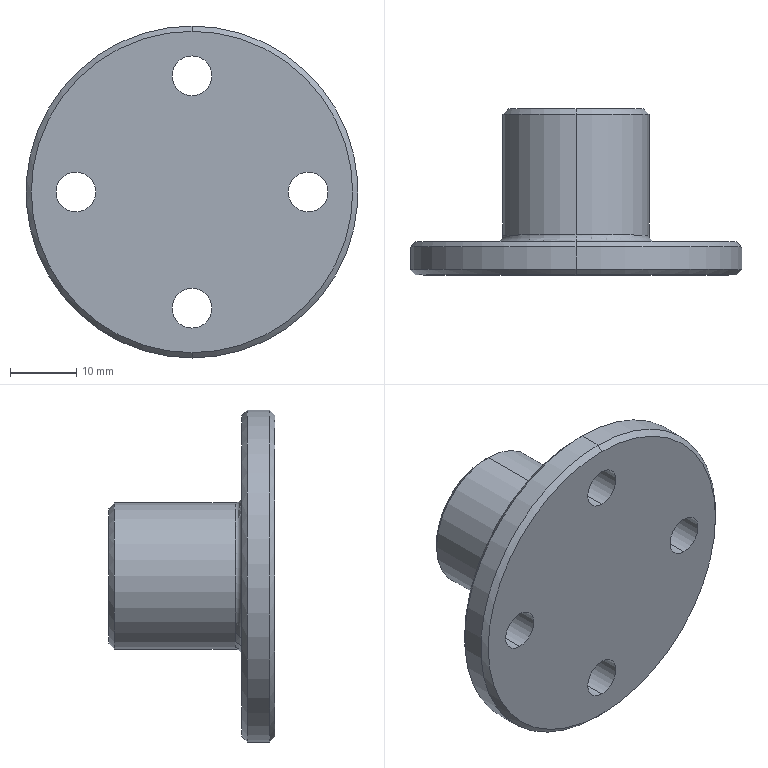Part | SolidWorks | features ICE 2, Chamfer 1, Extrusion 1, Fillet 1 | 1 solid | 28 faces | box 50 x 25 x 50 mm | volume 12711 mm3 | cylinder 14 | cone 8 | plane 4 | torus 2 | commonest cylinder face diameters 6 x8 16 x2 22 x2 50 x2
STEP:
#1=CARTESIAN_POINT('',(0.,6.,-11.));
#2=VERTEX_POINT('',#1);
#3=CARTESIAN_POINT('',(0.,6.,11.));
#4=VERTEX_POINT('',#3);
#5=CARTESIAN_POINT('',(0.,6.,0.));
#6=DIRECTION('',(0.,1.,0.));
#7=DIRECTION('',(0.,0.,1.));
#8=AXIS2_PLACEMENT_3D('',#5,#6,#7);
#9=CIRCLE('',#8,11.);
#10=EDGE_CURVE('',#2,#4,#9,.T.);
#11=ORIENTED_EDGE('',*,*,#10,.F.);
#12=CARTESIAN_POINT('',(0.,5.,-12.));
#13=VERTEX_POINT('',#12);
#14=CARTESIAN_POINT('',(0.,6.,-12.));
#15=DIRECTION('',(1.,0.,0.));
#16=DIRECTION('',(0.,0.,-1.));
#17=AXIS2_PLACEMENT_3D('',#14,#15,#16);
#18=CIRCLE('',#17,1.);
#19=EDGE_CURVE('',#2,#13,#18,.T.);
#20=ORIENTED_EDGE('',*,*,#19,.T.);
#21=CARTESIAN_POINT('',(0.,5.,12.));
#22=VERTEX_POINT('',#21);
#23=CARTESIAN_POINT('',(0.,5.,0.));
#24=DIRECTION('',(0.,-1.,0.));
#25=DIRECTION('',(0.,0.,1.));
#26=AXIS2_PLACEMENT_3D('',#23,#24,#25);
#27=CIRCLE('',#26,12.);
#28=EDGE_CURVE('',#22,#13,#27,.T.);
#29=ORIENTED_EDGE('',*,*,#28,.F.);
#30=CARTESIAN_POINT('',(0.,6.,12.));
#31=DIRECTION('',(-1.,0.,0.));
#32=DIRECTION('',(0.,0.,1.));
#33=AXIS2_PLACEMENT_3D('',#30,#31,#32);
#34=CIRCLE('',#33,1.);
#35=EDGE_CURVE('',#4,#22,#34,.T.);
#36=ORIENTED_EDGE('',*,*,#35,.F.);
#37=EDGE_LOOP('',(#11,#20,#29,#36));
#38=FACE_OUTER_BOUND('',#37,.T.);
#39=CARTESIAN_POINT('',(0.,6.,0.));
#40=DIRECTION('',(0.,1.,0.));
#41=DIRECTION('',(0.,0.,1.));
#42=AXIS2_PLACEMENT_3D('',#39,#40,#41);
#43=TOROIDAL_SURFACE('',#42,12.,1.);
#44=ADVANCED_FACE('',(#38),#43,.F.);
#45=CARTESIAN_POINT('',(0.,0.,-24.2));
#46=VERTEX_POINT('',#45);
#47=CARTESIAN_POINT('',(0.,0.,24.2));
#48=VERTEX_POINT('',#47);
#49=CARTESIAN_POINT('',(0.,0.,0.));
#50=DIRECTION('',(0.,-1.,0.));
#51=DIRECTION('',(0.,0.,1.));
#52=AXIS2_PLACEMENT_3D('',#49,#50,#51);
#53=CIRCLE('',#52,24.2);
#54=EDGE_CURVE('',#46,#48,#53,.T.);
#55=ORIENTED_EDGE('',*,*,#54,.F.);
#56=CARTESIAN_POINT('',(0.,0.8,-25.));
#57=VERTEX_POINT('',#56);
#58=CARTESIAN_POINT('',(0.,0.8,-25.));
#59=DIRECTION('',(0.,0.7071,-0.7071));
#60=VECTOR('',#59,1000.);
#61=LINE('',#58,#60);
#62=EDGE_CURVE('',#46,#57,#61,.T.);
#63=ORIENTED_EDGE('',*,*,#62,.T.);
#64=CARTESIAN_POINT('',(0.,0.8,25.));
#65=VERTEX_POINT('',#64);
#66=CARTESIAN_POINT('',(0.,0.8,0.));
#67=DIRECTION('',(0.,1.,0.));
#68=DIRECTION('',(0.,0.,1.));
#69=AXIS2_PLACEMENT_3D('',#66,#67,#68);
#70=CIRCLE('',#69,25.);
#71=EDGE_CURVE('',#65,#57,#70,.T.);
#72=ORIENTED_EDGE('',*,*,#71,.F.);
#73=CARTESIAN_POINT('',(0.,0.8,25.));
#74=DIRECTION('',(0.,0.7071,0.7071));
#75=VECTOR('',#74,1000.);
#76=LINE('',#73,#75);
#77=EDGE_CURVE('',#48,#65,#76,.T.);
#78=ORIENTED_EDGE('',*,*,#77,.F.);
#79=EDGE_LOOP('',(#55,#63,#72,#78));
#80=FACE_OUTER_BOUND('',#79,.T.);
#81=CARTESIAN_POINT('',(0.,0.8,0.));
#82=DIRECTION('',(0.,1.,0.));
#83=DIRECTION('',(0.,0.,1.));
#84=AXIS2_PLACEMENT_3D('',#81,#82,#83);
#85=CONICAL_SURFACE('',#84,25.,0.7854);
#86=ADVANCED_FACE('',(#80),#85,.T.);
#87=CARTESIAN_POINT('',(0.,5.,24.2));
#88=VERTEX_POINT('',#87);
#89=CARTESIAN_POINT('',(0.,5.,-24.2));
#90=VERTEX_POINT('',#89);
#91=CARTESIAN_POINT('',(0.,5.,0.));
#92=DIRECTION('',(0.,1.,0.));
#93=DIRECTION('',(0.,0.,1.));
#94=AXIS2_PLACEMENT_3D('',#91,#92,#93);
#95=CIRCLE('',#94,24.2);
#96=EDGE_CURVE('',#88,#90,#95,.T.);
#97=ORIENTED_EDGE('',*,*,#96,.F.);
#98=CARTESIAN_POINT('',(0.,4.2,25.));
#99=VERTEX_POINT('',#98);
#100=CARTESIAN_POINT('',(0.,5.,24.2));
#101=DIRECTION('',(0.,-0.7071,0.7071));
#102=VECTOR('',#101,1000.);
#103=LINE('',#100,#102);
#104=EDGE_CURVE('',#88,#99,#103,.T.);
#105=ORIENTED_EDGE('',*,*,#104,.T.);
#106=CARTESIAN_POINT('',(0.,4.2,-25.));
#107=VERTEX_POINT('',#106);
#108=CARTESIAN_POINT('',(0.,4.2,0.));
#109=DIRECTION('',(0.,-1.,0.));
#110=DIRECTION('',(0.,0.,1.));
#111=AXIS2_PLACEMENT_3D('',#108,#109,#110);
#112=CIRCLE('',#111,25.);
#113=EDGE_CURVE('',#107,#99,#112,.T.);
#114=ORIENTED_EDGE('',*,*,#113,.F.);
#115=CARTESIAN_POINT('',(0.,5.,-24.2));
#116=DIRECTION('',(0.,-0.7071,-0.7071));
#117=VECTOR('',#116,1000.);
#118=LINE('',#115,#117);
#119=EDGE_CURVE('',#90,#107,#118,.T.);
#120=ORIENTED_EDGE('',*,*,#119,.F.);
#121=EDGE_LOOP('',(#97,#105,#114,#120));
#122=FACE_OUTER_BOUND('',#121,.T.);
#123=CARTESIAN_POINT('',(0.,5.,0.));
#124=DIRECTION('',(0.,-1.,0.));
#125=DIRECTION('',(0.,0.,-1.));
#126=AXIS2_PLACEMENT_3D('',#123,#124,#125);
#127=CONICAL_SURFACE('',#126,24.2,0.7854);
#128=ADVANCED_FACE('',(#122),#127,.T.);
#129=CARTESIAN_POINT('',(0.,24.2,-8.));
#130=VERTEX_POINT('',#129);
#131=CARTESIAN_POINT('',(0.,24.2,8.));
#132=VERTEX_POINT('',#131);
#133=CARTESIAN_POINT('',(0.,24.2,0.));
#134=DIRECTION('',(0.,1.,0.));
#135=DIRECTION('',(0.,0.,1.));
#136=AXIS2_PLACEMENT_3D('',#133,#134,#135);
#137=CIRCLE('',#136,8.);
#138=EDGE_CURVE('',#130,#132,#137,.T.);
#139=ORIENTED_EDGE('',*,*,#138,.F.);
#140=CARTESIAN_POINT('',(0.,25.,-8.8));
#141=VERTEX_POINT('',#140);
#142=CARTESIAN_POINT('',(0.,24.2,-8.));
#143=DIRECTION('',(0.,0.7071,-0.7071));
#144=VECTOR('',#143,1000.);
#145=LINE('',#142,#144);
#146=EDGE_CURVE('',#130,#141,#145,.T.);
#147=ORIENTED_EDGE('',*,*,#146,.T.);
#148=CARTESIAN_POINT('',(0.,25.,8.8));
#149=VERTEX_POINT('',#148);
#150=CARTESIAN_POINT('',(0.,25.,0.));
#151=DIRECTION('',(0.,-1.,0.));
#152=DIRECTION('',(0.,0.,1.));
#153=AXIS2_PLACEMENT_3D('',#150,#151,#152);
#154=CIRCLE('',#153,8.8);
#155=EDGE_CURVE('',#149,#141,#154,.T.);
#156=ORIENTED_EDGE('',*,*,#155,.F.);
#157=CARTESIAN_POINT('',(0.,24.2,8.));
#158=DIRECTION('',(0.,0.7071,0.7071));
#159=VECTOR('',#158,1000.);
#160=LINE('',#157,#159);
#161=EDGE_CURVE('',#132,#149,#160,.T.);
#162=ORIENTED_EDGE('',*,*,#161,.F.);
#163=EDGE_LOOP('',(#139,#147,#156,#162));
#164=FACE_OUTER_BOUND('',#163,.T.);
#165=CARTESIAN_POINT('',(0.,24.2,0.));
#166=DIRECTION('',(0.,1.,0.));
#167=DIRECTION('',(0.,0.,1.));
#168=AXIS2_PLACEMENT_3D('',#165,#166,#167);
#169=CONICAL_SURFACE('',#168,8.,0.7854);
#170=ADVANCED_FACE('',(#164),#169,.F.);
#171=CARTESIAN_POINT('',(0.,25.,10.2));
#172=VERTEX_POINT('',#171);
#173=CARTESIAN_POINT('',(0.,25.,-10.2));
#174=VERTEX_POINT('',#173);
#175=CARTESIAN_POINT('',(0.,25.,0.));
#176=DIRECTION('',(0.,1.,0.));
#177=DIRECTION('',(0.,0.,1.));
#178=AXIS2_PLACEMENT_3D('',#175,#176,#177);
#179=CIRCLE('',#178,10.2);
#180=EDGE_CURVE('',#172,#174,#179,.T.);
#181=ORIENTED_EDGE('',*,*,#180,.F.);
#182=CARTESIAN_POINT('',(0.,24.2,11.));
#183=VERTEX_POINT('',#182);
#184=CARTESIAN_POINT('',(0.,25.,10.2));
#185=DIRECTION('',(0.,-0.7071,0.7071));
#186=VECTOR('',#185,1000.);
#187=LINE('',#184,#186);
#188=EDGE_CURVE('',#172,#183,#187,.T.);
#189=ORIENTED_EDGE('',*,*,#188,.T.);
#190=CARTESIAN_POINT('',(0.,24.2,-11.));
#191=VERTEX_POINT('',#190);
#192=CARTESIAN_POINT('',(0.,24.2,0.));
#193=DIRECTION('',(0.,-1.,0.));
#194=DIRECTION('',(0.,0.,1.));
#195=AXIS2_PLACEMENT_3D('',#192,#193,#194);
#196=CIRCLE('',#195,11.);
#197=EDGE_CURVE('',#191,#183,#196,.T.);
#198=ORIENTED_EDGE('',*,*,#197,.F.);
#199=CARTESIAN_POINT('',(0.,25.,-10.2));
#200=DIRECTION('',(0.,-0.7071,-0.7071));
#201=VECTOR('',#200,1000.);
#202=LINE('',#199,#201);
#203=EDGE_CURVE('',#174,#191,#202,.T.);
#204=ORIENTED_EDGE('',*,*,#203,.F.);
#205=EDGE_LOOP('',(#181,#189,#198,#204));
#206=FACE_OUTER_BOUND('',#205,.T.);
#207=CARTESIAN_POINT('',(0.,25.,0.));
#208=DIRECTION('',(0.,-1.,0.));
#209=DIRECTION('',(0.,0.,-1.));
#210=AXIS2_PLACEMENT_3D('',#207,#208,#209);
#211=CONICAL_SURFACE('',#210,10.2,0.7854);
#212=ADVANCED_FACE('',(#206),#211,.T.);
#213=ORIENTED_EDGE('',*,*,#138,.T.);
#214=CARTESIAN_POINT('',(0.,5.,8.));
#215=VERTEX_POINT('',#214);
#216=CARTESIAN_POINT('',(0.,25.,8.));
#217=DIRECTION('',(0.,-1.,0.));
#218=VECTOR('',#217,1000.);
#219=LINE('',#216,#218);
#220=EDGE_CURVE('',#132,#215,#219,.T.);
#221=ORIENTED_EDGE('',*,*,#220,.T.);
#222=CARTESIAN_POINT('',(0.,5.,-8.));
#223=VERTEX_POINT('',#222);
#224=CARTESIAN_POINT('',(0.,5.,0.));
#225=DIRECTION('',(0.,-1.,0.));
#226=DIRECTION('',(0.,0.,1.));
#227=AXIS2_PLACEMENT_3D('',#224,#225,#226);
#228=CIRCLE('',#227,8.);
#229=EDGE_CURVE('',#215,#223,#228,.T.);
#230=ORIENTED_EDGE('',*,*,#229,.T.);
#231=CARTESIAN_POINT('',(0.,25.,-8.));
#232=DIRECTION('',(0.,-1.,0.));
#233=VECTOR('',#232,1000.);
#234=LINE('',#231,#233);
#235=EDGE_CURVE('',#130,#223,#234,.T.);
#236=ORIENTED_EDGE('',*,*,#235,.F.);
#237=EDGE_LOOP('',(#213,#221,#230,#236));
#238=FACE_OUTER_BOUND('',#237,.T.);
#239=CARTESIAN_POINT('',(0.,25.,0.));
#240=DIRECTION('',(0.,-1.,0.));
#241=DIRECTION('',(0.,0.,-1.));
#242=AXIS2_PLACEMENT_3D('',#239,#240,#241);
#243=CYLINDRICAL_SURFACE('',#242,8.);
#244=ADVANCED_FACE('',(#238),#243,.F.);
#245=ORIENTED_EDGE('',*,*,#197,.T.);
#246=CARTESIAN_POINT('',(0.,25.,11.));
#247=DIRECTION('',(0.,-1.,0.));
#248=VECTOR('',#247,1000.);
#249=LINE('',#246,#248);
#250=EDGE_CURVE('',#183,#4,#249,.T.);
#251=ORIENTED_EDGE('',*,*,#250,.T.);
#252=CARTESIAN_POINT('',(0.,6.,0.));
#253=DIRECTION('',(0.,1.,0.));
#254=DIRECTION('',(0.,0.,1.));
#255=AXIS2_PLACEMENT_3D('',#252,#253,#254);
#256=CIRCLE('',#255,11.);
#257=EDGE_CURVE('',#4,#2,#256,.T.);
#258=ORIENTED_EDGE('',*,*,#257,.T.);
#259=CARTESIAN_POINT('',(0.,25.,-11.));
#260=DIRECTION('',(0.,-1.,0.));
#261=VECTOR('',#260,1000.);
#262=LINE('',#259,#261);
#263=EDGE_CURVE('',#191,#2,#262,.T.);
#264=ORIENTED_EDGE('',*,*,#263,.F.);
#265=EDGE_LOOP('',(#245,#251,#258,#264));
#266=FACE_OUTER_BOUND('',#265,.T.);
#267=CARTESIAN_POINT('',(0.,25.,0.));
#268=DIRECTION('',(0.,-1.,0.));
#269=DIRECTION('',(0.,0.,-1.));
#270=AXIS2_PLACEMENT_3D('',#267,#268,#269);
#271=CYLINDRICAL_SURFACE('',#270,11.);
#272=ADVANCED_FACE('',(#266),#271,.T.);
#273=CARTESIAN_POINT('',(-17.5,5.,-3.));
#274=VERTEX_POINT('',#273);
#275=CARTESIAN_POINT('',(-17.5,5.,3.));
#276=VERTEX_POINT('',#275);
#277=CARTESIAN_POINT('',(-17.5,5.,0.));
#278=DIRECTION('',(0.,1.,0.));
#279=DIRECTION('',(0.,0.,1.));
#280=AXIS2_PLACEMENT_3D('',#277,#278,#279);
#281=CIRCLE('',#280,3.);
#282=EDGE_CURVE('',#274,#276,#281,.T.);
#283=ORIENTED_EDGE('',*,*,#282,.T.);
#284=CARTESIAN_POINT('',(-17.5,0.,3.));
#285=VERTEX_POINT('',#284);
#286=CARTESIAN_POINT('',(-17.5,5.,3.));
#287=DIRECTION('',(0.,-1.,0.));
#288=VECTOR('',#287,1000.);
#289=LINE('',#286,#288);
#290=EDGE_CURVE('',#276,#285,#289,.T.);
#291=ORIENTED_EDGE('',*,*,#290,.T.);
#292=CARTESIAN_POINT('',(-17.5,0.,-3.));
#293=VERTEX_POINT('',#292);
#294=CARTESIAN_POINT('',(-17.5,0.,0.));
#295=DIRECTION('',(0.,1.,0.));
#296=DIRECTION('',(0.,0.,1.));
#297=AXIS2_PLACEMENT_3D('',#294,#295,#296);
#298=CIRCLE('',#297,3.);
#299=EDGE_CURVE('',#293,#285,#298,.T.);
#300=ORIENTED_EDGE('',*,*,#299,.F.);
#301=CARTESIAN_POINT('',(-17.5,5.,-3.));
#302=DIRECTION('',(0.,-1.,0.));
#303=VECTOR('',#302,1000.);
#304=LINE('',#301,#303);
#305=EDGE_CURVE('',#274,#293,#304,.T.);
#306=ORIENTED_EDGE('',*,*,#305,.F.);
#307=EDGE_LOOP('',(#283,#291,#300,#306));
#308=FACE_OUTER_BOUND('',#307,.T.);
#309=CARTESIAN_POINT('',(-17.5,5.,0.));
#310=DIRECTION('',(0.,-1.,0.));
#311=DIRECTION('',(0.,0.,-1.));
#312=AXIS2_PLACEMENT_3D('',#309,#310,#311);
#313=CYLINDRICAL_SURFACE('',#312,3.);
#314=ADVANCED_FACE('',(#308),#313,.F.);
#315=CARTESIAN_POINT('',(0.,5.,-20.5));
#316=VERTEX_POINT('',#315);
#317=CARTESIAN_POINT('',(0.,5.,-14.5));
#318=VERTEX_POINT('',#317);
#319=CARTESIAN_POINT('',(0.,5.,-17.5));
#320=DIRECTION('',(0.,1.,0.));
#321=DIRECTION('',(0.,0.,1.));
#322=AXIS2_PLACEMENT_3D('',#319,#320,#321);
#323=CIRCLE('',#322,3.);
#324=EDGE_CURVE('',#316,#318,#323,.T.);
#325=ORIENTED_EDGE('',*,*,#324,.T.);
#326=CARTESIAN_POINT('',(0.,0.,-14.5));
#327=VERTEX_POINT('',#326);
#328=CARTESIAN_POINT('',(0.,5.,-14.5));
#329=DIRECTION('',(0.,-1.,0.));
#330=VECTOR('',#329,1000.);
#331=LINE('',#328,#330);
#332=EDGE_CURVE('',#318,#327,#331,.T.);
#333=ORIENTED_EDGE('',*,*,#332,.T.);
#334=CARTESIAN_POINT('',(0.,0.,-20.5));
#335=VERTEX_POINT('',#334);
#336=CARTESIAN_POINT('',(0.,0.,-17.5));
#337=DIRECTION('',(0.,1.,0.));
#338=DIRECTION('',(0.,0.,1.));
#339=AXIS2_PLACEMENT_3D('',#336,#337,#338);
#340=CIRCLE('',#339,3.);
#341=EDGE_CURVE('',#335,#327,#340,.T.);
#342=ORIENTED_EDGE('',*,*,#341,.F.);
#343=CARTESIAN_POINT('',(0.,5.,-20.5));
#344=DIRECTION('',(0.,-1.,0.));
#345=VECTOR('',#344,1000.);
#346=LINE('',#343,#345);
#347=EDGE_CURVE('',#316,#335,#346,.T.);
#348=ORIENTED_EDGE('',*,*,#347,.F.);
#349=EDGE_LOOP('',(#325,#333,#342,#348));
#350=FACE_OUTER_BOUND('',#349,.T.);
#351=CARTESIAN_POINT('',(0.,5.,-17.5));
#352=DIRECTION('',(0.,-1.,0.));
#353=DIRECTION('',(0.,0.,-1.));
#354=AXIS2_PLACEMENT_3D('',#351,#352,#353);
#355=CYLINDRICAL_SURFACE('',#354,3.);
#356=ADVANCED_FACE('',(#350),#355,.F.);
#357=CARTESIAN_POINT('',(17.5,5.,-3.));
#358=VERTEX_POINT('',#357);
#359=CARTESIAN_POINT('',(17.5,5.,3.));
#360=VERTEX_POINT('',#359);
#361=CARTESIAN_POINT('',(17.5,5.,0.));
#362=DIRECTION('',(0.,1.,0.));
#363=DIRECTION('',(0.,0.,1.));
#364=AXIS2_PLACEMENT_3D('',#361,#362,#363);
#365=CIRCLE('',#364,3.);
#366=EDGE_CURVE('',#358,#360,#365,.T.);
#367=ORIENTED_EDGE('',*,*,#366,.T.);
#368=CARTESIAN_POINT('',(17.5,0.,3.));
#369=VERTEX_POINT('',#368);
#370=CARTESIAN_POINT('',(17.5,5.,3.));
#371=DIRECTION('',(0.,-1.,0.));
#372=VECTOR('',#371,1000.);
#373=LINE('',#370,#372);
#374=EDGE_CURVE('',#360,#369,#373,.T.);
#375=ORIENTED_EDGE('',*,*,#374,.T.);
#376=CARTESIAN_POINT('',(17.5,0.,-3.));
#377=VERTEX_POINT('',#376);
#378=CARTESIAN_POINT('',(17.5,0.,0.));
#379=DIRECTION('',(0.,1.,0.));
#380=DIRECTION('',(0.,0.,1.));
#381=AXIS2_PLACEMENT_3D('',#378,#379,#380);
#382=CIRCLE('',#381,3.);
#383=EDGE_CURVE('',#377,#369,#382,.T.);
#384=ORIENTED_EDGE('',*,*,#383,.F.);
#385=CARTESIAN_POINT('',(17.5,5.,-3.));
#386=DIRECTION('',(0.,-1.,0.));
#387=VECTOR('',#386,1000.);
#388=LINE('',#385,#387);
#389=EDGE_CURVE('',#358,#377,#388,.T.);
#390=ORIENTED_EDGE('',*,*,#389,.F.);
#391=EDGE_LOOP('',(#367,#375,#384,#390));
#392=FACE_OUTER_BOUND('',#391,.T.);
#393=CARTESIAN_POINT('',(17.5,5.,0.));
#394=DIRECTION('',(0.,-1.,0.));
#395=DIRECTION('',(0.,0.,-1.));
#396=AXIS2_PLACEMENT_3D('',#393,#394,#395);
#397=CYLINDRICAL_SURFACE('',#396,3.);
#398=ADVANCED_FACE('',(#392),#397,.F.);
#399=CARTESIAN_POINT('',(0.,5.,14.5));
#400=VERTEX_POINT('',#399);
#401=CARTESIAN_POINT('',(0.,5.,20.5));
#402=VERTEX_POINT('',#401);
#403=CARTESIAN_POINT('',(0.,5.,17.5));
#404=DIRECTION('',(0.,1.,0.));
#405=DIRECTION('',(0.,0.,1.));
#406=AXIS2_PLACEMENT_3D('',#403,#404,#405);
#407=CIRCLE('',#406,3.);
#408=EDGE_CURVE('',#400,#402,#407,.T.);
#409=ORIENTED_EDGE('',*,*,#408,.T.);
#410=CARTESIAN_POINT('',(0.,0.,20.5));
#411=VERTEX_POINT('',#410);
#412=CARTESIAN_POINT('',(0.,5.,20.5));
#413=DIRECTION('',(0.,-1.,0.));
#414=VECTOR('',#413,1000.);
#415=LINE('',#412,#414);
#416=EDGE_CURVE('',#402,#411,#415,.T.);
#417=ORIENTED_EDGE('',*,*,#416,.T.);
#418=CARTESIAN_POINT('',(0.,0.,14.5));
#419=VERTEX_POINT('',#418);
#420=CARTESIAN_POINT('',(0.,0.,17.5));
#421=DIRECTION('',(0.,1.,0.));
#422=DIRECTION('',(0.,0.,1.));
#423=AXIS2_PLACEMENT_3D('',#420,#421,#422);
#424=CIRCLE('',#423,3.);
#425=EDGE_CURVE('',#419,#411,#424,.T.);
#426=ORIENTED_EDGE('',*,*,#425,.F.);
#427=CARTESIAN_POINT('',(0.,5.,14.5));
#428=DIRECTION('',(0.,-1.,0.));
#429=VECTOR('',#428,1000.);
#430=LINE('',#427,#429);
#431=EDGE_CURVE('',#400,#419,#430,.T.);
#432=ORIENTED_EDGE('',*,*,#431,.F.);
#433=EDGE_LOOP('',(#409,#417,#426,#432));
#434=FACE_OUTER_BOUND('',#433,.T.);
#435=CARTESIAN_POINT('',(0.,5.,17.5));
#436=DIRECTION('',(0.,-1.,0.));
#437=DIRECTION('',(0.,0.,-1.));
#438=AXIS2_PLACEMENT_3D('',#435,#436,#437);
#439=CYLINDRICAL_SURFACE('',#438,3.);
#440=ADVANCED_FACE('',(#434),#439,.F.);
#441=ORIENTED_EDGE('',*,*,#113,.T.);
#442=CARTESIAN_POINT('',(0.,5.,25.));
#443=DIRECTION('',(0.,-1.,0.));
#444=VECTOR('',#443,1000.);
#445=LINE('',#442,#444);
#446=EDGE_CURVE('',#99,#65,#445,.T.);
#447=ORIENTED_EDGE('',*,*,#446,.T.);
#448=ORIENTED_EDGE('',*,*,#71,.T.);
#449=CARTESIAN_POINT('',(0.,5.,-25.));
#450=DIRECTION('',(0.,-1.,0.));
#451=VECTOR('',#450,1000.);
#452=LINE('',#449,#451);
#453=EDGE_CURVE('',#107,#57,#452,.T.);
#454=ORIENTED_EDGE('',*,*,#453,.F.);
#455=EDGE_LOOP('',(#441,#447,#448,#454));
#456=FACE_OUTER_BOUND('',#455,.T.);
#457=CARTESIAN_POINT('',(0.,5.,0.));
#458=DIRECTION('',(0.,-1.,0.));
#459=DIRECTION('',(0.,0.,-1.));
#460=AXIS2_PLACEMENT_3D('',#457,#458,#459);
#461=CYLINDRICAL_SURFACE('',#460,25.);
#462=ADVANCED_FACE('',(#456),#461,.T.);
#463=ORIENTED_EDGE('',*,*,#446,.F.);
#464=CARTESIAN_POINT('',(0.,4.2,0.));
#465=DIRECTION('',(0.,-1.,0.));
#466=DIRECTION('',(0.,0.,1.));
#467=AXIS2_PLACEMENT_3D('',#464,#465,#466);
#468=CIRCLE('',#467,25.);
#469=EDGE_CURVE('',#99,#107,#468,.T.);
#470=ORIENTED_EDGE('',*,*,#469,.T.);
#471=ORIENTED_EDGE('',*,*,#453,.T.);
#472=CARTESIAN_POINT('',(0.,0.8,0.));
#473=DIRECTION('',(0.,1.,0.));
#474=DIRECTION('',(0.,0.,1.));
#475=AXIS2_PLACEMENT_3D('',#472,#473,#474);
#476=CIRCLE('',#475,25.);
#477=EDGE_CURVE('',#57,#65,#476,.T.);
#478=ORIENTED_EDGE('',*,*,#477,.T.);
#479=EDGE_LOOP('',(#463,#470,#471,#478));
#480=FACE_OUTER_BOUND('',#479,.T.);
#481=CARTESIAN_POINT('',(0.,5.,0.));
#482=DIRECTION('',(0.,-1.,0.));
#483=DIRECTION('',(0.,0.,-1.));
#484=AXIS2_PLACEMENT_3D('',#481,#482,#483);
#485=CYLINDRICAL_SURFACE('',#484,25.);
#486=ADVANCED_FACE('',(#480),#485,.T.);
#487=ORIENTED_EDGE('',*,*,#28,.T.);
#488=CARTESIAN_POINT('',(0.,5.,0.));
#489=DIRECTION('',(0.,-1.,0.));
#490=DIRECTION('',(0.,0.,1.));
#491=AXIS2_PLACEMENT_3D('',#488,#489,#490);
#492=CIRCLE('',#491,12.);
#493=EDGE_CURVE('',#13,#22,#492,.T.);
#494=ORIENTED_EDGE('',*,*,#493,.T.);
#495=EDGE_LOOP('',(#487,#494));
#496=FACE_BOUND('',#495,.T.);
#497=CARTESIAN_POINT('',(0.,5.,0.));
#498=DIRECTION('',(0.,1.,0.));
#499=DIRECTION('',(0.,0.,1.));
#500=AXIS2_PLACEMENT_3D('',#497,#498,#499);
#501=CIRCLE('',#500,24.2);
#502=EDGE_CURVE('',#90,#88,#501,.T.);
#503=ORIENTED_EDGE('',*,*,#502,.T.);
#504=ORIENTED_EDGE('',*,*,#96,.T.);
#505=EDGE_LOOP('',(#503,#504));
#506=FACE_OUTER_BOUND('',#505,.T.);
#507=ORIENTED_EDGE('',*,*,#282,.F.);
#508=CARTESIAN_POINT('',(-17.5,5.,0.));
#509=DIRECTION('',(0.,1.,0.));
#510=DIRECTION('',(0.,0.,1.));
#511=AXIS2_PLACEMENT_3D('',#508,#509,#510);
#512=CIRCLE('',#511,3.);
#513=EDGE_CURVE('',#276,#274,#512,.T.);
#514=ORIENTED_EDGE('',*,*,#513,.F.);
#515=EDGE_LOOP('',(#507,#514));
#516=FACE_BOUND('',#515,.T.);
#517=ORIENTED_EDGE('',*,*,#324,.F.);
#518=CARTESIAN_POINT('',(0.,5.,-17.5));
#519=DIRECTION('',(0.,1.,0.));
#520=DIRECTION('',(0.,0.,1.));
#521=AXIS2_PLACEMENT_3D('',#518,#519,#520);
#522=CIRCLE('',#521,3.);
#523=EDGE_CURVE('',#318,#316,#522,.T.);
#524=ORIENTED_EDGE('',*,*,#523,.F.);
#525=EDGE_LOOP('',(#517,#524));
#526=FACE_BOUND('',#525,.T.);
#527=ORIENTED_EDGE('',*,*,#366,.F.);
#528=CARTESIAN_POINT('',(17.5,5.,0.));
#529=DIRECTION('',(0.,1.,0.));
#530=DIRECTION('',(0.,0.,1.));
#531=AXIS2_PLACEMENT_3D('',#528,#529,#530);
#532=CIRCLE('',#531,3.);
#533=EDGE_CURVE('',#360,#358,#532,.T.);
#534=ORIENTED_EDGE('',*,*,#533,.F.);
#535=EDGE_LOOP('',(#527,#534));
#536=FACE_BOUND('',#535,.T.);
#537=ORIENTED_EDGE('',*,*,#408,.F.);
#538=CARTESIAN_POINT('',(0.,5.,17.5));
#539=DIRECTION('',(0.,1.,0.));
#540=DIRECTION('',(0.,0.,1.));
#541=AXIS2_PLACEMENT_3D('',#538,#539,#540);
#542=CIRCLE('',#541,3.);
#543=EDGE_CURVE('',#402,#400,#542,.T.);
#544=ORIENTED_EDGE('',*,*,#543,.F.);
#545=EDGE_LOOP('',(#537,#544));
#546=FACE_BOUND('',#545,.T.);
#547=CARTESIAN_POINT('',(0.,5.,0.));
#548=DIRECTION('',(0.,1.,0.));
#549=DIRECTION('',(0.,0.,1.));
#550=AXIS2_PLACEMENT_3D('',#547,#548,#549);
#551=PLANE('',#550);
#552=ADVANCED_FACE('',(#496,#506,#516,#526,#536,#546),#551,.T.);
#553=CARTESIAN_POINT('',(0.,0.,0.));
#554=DIRECTION('',(0.,-1.,0.));
#555=DIRECTION('',(0.,0.,1.));
#556=AXIS2_PLACEMENT_3D('',#553,#554,#555);
#557=CIRCLE('',#556,24.2);
#558=EDGE_CURVE('',#48,#46,#557,.T.);
#559=ORIENTED_EDGE('',*,*,#558,.T.);
#560=ORIENTED_EDGE('',*,*,#54,.T.);
#561=EDGE_LOOP('',(#559,#560));
#562=FACE_OUTER_BOUND('',#561,.T.);
#563=ORIENTED_EDGE('',*,*,#299,.T.);
#564=CARTESIAN_POINT('',(-17.5,0.,0.));
#565=DIRECTION('',(0.,1.,0.));
#566=DIRECTION('',(0.,0.,1.));
#567=AXIS2_PLACEMENT_3D('',#564,#565,#566);
#568=CIRCLE('',#567,3.);
#569=EDGE_CURVE('',#285,#293,#568,.T.);
#570=ORIENTED_EDGE('',*,*,#569,.T.);
#571=EDGE_LOOP('',(#563,#570));
#572=FACE_BOUND('',#571,.T.);
#573=ORIENTED_EDGE('',*,*,#341,.T.);
#574=CARTESIAN_POINT('',(0.,0.,-17.5));
#575=DIRECTION('',(0.,1.,0.));
#576=DIRECTION('',(0.,0.,1.));
#577=AXIS2_PLACEMENT_3D('',#574,#575,#576);
#578=CIRCLE('',#577,3.);
#579=EDGE_CURVE('',#327,#335,#578,.T.);
#580=ORIENTED_EDGE('',*,*,#579,.T.);
#581=EDGE_LOOP('',(#573,#580));
#582=FACE_BOUND('',#581,.T.);
#583=ORIENTED_EDGE('',*,*,#383,.T.);
#584=CARTESIAN_POINT('',(17.5,0.,0.));
#585=DIRECTION('',(0.,1.,0.));
#586=DIRECTION('',(0.,0.,1.));
#587=AXIS2_PLACEMENT_3D('',#584,#585,#586);
#588=CIRCLE('',#587,3.);
#589=EDGE_CURVE('',#369,#377,#588,.T.);
#590=ORIENTED_EDGE('',*,*,#589,.T.);
#591=EDGE_LOOP('',(#583,#590));
#592=FACE_BOUND('',#591,.T.);
#593=ORIENTED_EDGE('',*,*,#425,.T.);
#594=CARTESIAN_POINT('',(0.,0.,17.5));
#595=DIRECTION('',(0.,1.,0.));
#596=DIRECTION('',(0.,0.,1.));
#597=AXIS2_PLACEMENT_3D('',#594,#595,#596);
#598=CIRCLE('',#597,3.);
#599=EDGE_CURVE('',#411,#419,#598,.T.);
#600=ORIENTED_EDGE('',*,*,#599,.T.);
#601=EDGE_LOOP('',(#593,#600));
#602=FACE_BOUND('',#601,.T.);
#603=CARTESIAN_POINT('',(0.,0.,0.));
#604=DIRECTION('',(0.,1.,0.));
#605=DIRECTION('',(0.,0.,1.));
#606=AXIS2_PLACEMENT_3D('',#603,#604,#605);
#607=PLANE('',#606);
#608=ADVANCED_FACE('',(#562,#572,#582,#592,#602),#607,.F.);
#609=ORIENTED_EDGE('',*,*,#416,.F.);
#610=ORIENTED_EDGE('',*,*,#543,.T.);
#611=ORIENTED_EDGE('',*,*,#431,.T.);
#612=ORIENTED_EDGE('',*,*,#599,.F.);
#613=EDGE_LOOP('',(#609,#610,#611,#612));
#614=FACE_OUTER_BOUND('',#613,.T.);
#615=CARTESIAN_POINT('',(0.,5.,17.5));
#616=DIRECTION('',(0.,-1.,0.));
#617=DIRECTION('',(0.,0.,-1.));
#618=AXIS2_PLACEMENT_3D('',#615,#616,#617);
#619=CYLINDRICAL_SURFACE('',#618,3.);
#620=ADVANCED_FACE('',(#614),#619,.F.);
#621=ORIENTED_EDGE('',*,*,#374,.F.);
#622=ORIENTED_EDGE('',*,*,#533,.T.);
#623=ORIENTED_EDGE('',*,*,#389,.T.);
#624=ORIENTED_EDGE('',*,*,#589,.F.);
#625=EDGE_LOOP('',(#621,#622,#623,#624));
#626=FACE_OUTER_BOUND('',#625,.T.);
#627=CARTESIAN_POINT('',(17.5,5.,0.));
#628=DIRECTION('',(0.,-1.,0.));
#629=DIRECTION('',(0.,0.,-1.));
#630=AXIS2_PLACEMENT_3D('',#627,#628,#629);
#631=CYLINDRICAL_SURFACE('',#630,3.);
#632=ADVANCED_FACE('',(#626),#631,.F.);
#633=ORIENTED_EDGE('',*,*,#332,.F.);
#634=ORIENTED_EDGE('',*,*,#523,.T.);
#635=ORIENTED_EDGE('',*,*,#347,.T.);
#636=ORIENTED_EDGE('',*,*,#579,.F.);
#637=EDGE_LOOP('',(#633,#634,#635,#636));
#638=FACE_OUTER_BOUND('',#637,.T.);
#639=CARTESIAN_POINT('',(0.,5.,-17.5));
#640=DIRECTION('',(0.,-1.,0.));
#641=DIRECTION('',(0.,0.,-1.));
#642=AXIS2_PLACEMENT_3D('',#639,#640,#641);
#643=CYLINDRICAL_SURFACE('',#642,3.);
#644=ADVANCED_FACE('',(#638),#643,.F.);
#645=ORIENTED_EDGE('',*,*,#290,.F.);
#646=ORIENTED_EDGE('',*,*,#513,.T.);
#647=ORIENTED_EDGE('',*,*,#305,.T.);
#648=ORIENTED_EDGE('',*,*,#569,.F.);
#649=EDGE_LOOP('',(#645,#646,#647,#648));
#650=FACE_OUTER_BOUND('',#649,.T.);
#651=CARTESIAN_POINT('',(-17.5,5.,0.));
#652=DIRECTION('',(0.,-1.,0.));
#653=DIRECTION('',(0.,0.,-1.));
#654=AXIS2_PLACEMENT_3D('',#651,#652,#653);
#655=CYLINDRICAL_SURFACE('',#654,3.);
#656=ADVANCED_FACE('',(#650),#655,.F.);
#657=CARTESIAN_POINT('',(0.,25.,0.));
#658=DIRECTION('',(0.,1.,0.));
#659=DIRECTION('',(0.,0.,1.));
#660=AXIS2_PLACEMENT_3D('',#657,#658,#659);
#661=CIRCLE('',#660,10.2);
#662=EDGE_CURVE('',#174,#172,#661,.T.);
#663=ORIENTED_EDGE('',*,*,#662,.T.);
#664=ORIENTED_EDGE('',*,*,#180,.T.);
#665=EDGE_LOOP('',(#663,#664));
#666=FACE_OUTER_BOUND('',#665,.T.);
#667=ORIENTED_EDGE('',*,*,#155,.T.);
#668=CARTESIAN_POINT('',(0.,25.,0.));
#669=DIRECTION('',(0.,-1.,0.));
#670=DIRECTION('',(0.,0.,1.));
#671=AXIS2_PLACEMENT_3D('',#668,#669,#670);
#672=CIRCLE('',#671,8.8);
#673=EDGE_CURVE('',#141,#149,#672,.T.);
#674=ORIENTED_EDGE('',*,*,#673,.T.);
#675=EDGE_LOOP('',(#667,#674));
#676=FACE_BOUND('',#675,.T.);
#677=CARTESIAN_POINT('',(0.,25.,0.));
#678=DIRECTION('',(0.,1.,0.));
#679=DIRECTION('',(0.,0.,1.));
#680=AXIS2_PLACEMENT_3D('',#677,#678,#679);
#681=PLANE('',#680);
#682=ADVANCED_FACE('',(#666,#676),#681,.T.);
#683=ORIENTED_EDGE('',*,*,#250,.F.);
#684=CARTESIAN_POINT('',(0.,24.2,0.));
#685=DIRECTION('',(0.,-1.,0.));
#686=DIRECTION('',(0.,0.,1.));
#687=AXIS2_PLACEMENT_3D('',#684,#685,#686);
#688=CIRCLE('',#687,11.);
#689=EDGE_CURVE('',#183,#191,#688,.T.);
#690=ORIENTED_EDGE('',*,*,#689,.T.);
#691=ORIENTED_EDGE('',*,*,#263,.T.);
#692=ORIENTED_EDGE('',*,*,#10,.T.);
#693=EDGE_LOOP('',(#683,#690,#691,#692));
#694=FACE_OUTER_BOUND('',#693,.T.);
#695=CARTESIAN_POINT('',(0.,25.,0.));
#696=DIRECTION('',(0.,-1.,0.));
#697=DIRECTION('',(0.,0.,-1.));
#698=AXIS2_PLACEMENT_3D('',#695,#696,#697);
#699=CYLINDRICAL_SURFACE('',#698,11.);
#700=ADVANCED_FACE('',(#694),#699,.T.);
#701=ORIENTED_EDGE('',*,*,#220,.F.);
#702=CARTESIAN_POINT('',(0.,24.2,0.));
#703=DIRECTION('',(0.,1.,0.));
#704=DIRECTION('',(0.,0.,1.));
#705=AXIS2_PLACEMENT_3D('',#702,#703,#704);
#706=CIRCLE('',#705,8.);
#707=EDGE_CURVE('',#132,#130,#706,.T.);
#708=ORIENTED_EDGE('',*,*,#707,.T.);
#709=ORIENTED_EDGE('',*,*,#235,.T.);
#710=CARTESIAN_POINT('',(0.,5.,0.));
#711=DIRECTION('',(0.,-1.,0.));
#712=DIRECTION('',(0.,0.,1.));
#713=AXIS2_PLACEMENT_3D('',#710,#711,#712);
#714=CIRCLE('',#713,8.);
#715=EDGE_CURVE('',#223,#215,#714,.T.);
#716=ORIENTED_EDGE('',*,*,#715,.T.);
#717=EDGE_LOOP('',(#701,#708,#709,#716));
#718=FACE_OUTER_BOUND('',#717,.T.);
#719=CARTESIAN_POINT('',(0.,25.,0.));
#720=DIRECTION('',(0.,-1.,0.));
#721=DIRECTION('',(0.,0.,-1.));
#722=AXIS2_PLACEMENT_3D('',#719,#720,#721);
#723=CYLINDRICAL_SURFACE('',#722,8.);
#724=ADVANCED_FACE('',(#718),#723,.F.);
#725=ORIENTED_EDGE('',*,*,#715,.F.);
#726=ORIENTED_EDGE('',*,*,#229,.F.);
#727=EDGE_LOOP('',(#725,#726));
#728=FACE_OUTER_BOUND('',#727,.T.);
#729=CARTESIAN_POINT('',(0.,5.,0.));
#730=DIRECTION('',(0.,1.,0.));
#731=DIRECTION('',(0.,0.,1.));
#732=AXIS2_PLACEMENT_3D('',#729,#730,#731);
#733=PLANE('',#732);
#734=ADVANCED_FACE('',(#728),#733,.T.);
#735=ORIENTED_EDGE('',*,*,#188,.F.);
#736=ORIENTED_EDGE('',*,*,#662,.F.);
#737=ORIENTED_EDGE('',*,*,#203,.T.);
#738=ORIENTED_EDGE('',*,*,#689,.F.);
#739=EDGE_LOOP('',(#735,#736,#737,#738));
#740=FACE_OUTER_BOUND('',#739,.T.);
#741=CARTESIAN_POINT('',(0.,25.,0.));
#742=DIRECTION('',(0.,-1.,0.));
#743=DIRECTION('',(0.,0.,-1.));
#744=AXIS2_PLACEMENT_3D('',#741,#742,#743);
#745=CONICAL_SURFACE('',#744,10.2,0.7854);
#746=ADVANCED_FACE('',(#740),#745,.T.);
#747=ORIENTED_EDGE('',*,*,#146,.F.);
#748=ORIENTED_EDGE('',*,*,#707,.F.);
#749=ORIENTED_EDGE('',*,*,#161,.T.);
#750=ORIENTED_EDGE('',*,*,#673,.F.);
#751=EDGE_LOOP('',(#747,#748,#749,#750));
#752=FACE_OUTER_BOUND('',#751,.T.);
#753=CARTESIAN_POINT('',(0.,24.2,0.));
#754=DIRECTION('',(0.,1.,0.));
#755=DIRECTION('',(0.,0.,1.));
#756=AXIS2_PLACEMENT_3D('',#753,#754,#755);
#757=CONICAL_SURFACE('',#756,8.,0.7854);
#758=ADVANCED_FACE('',(#752),#757,.F.);
#759=ORIENTED_EDGE('',*,*,#104,.F.);
#760=ORIENTED_EDGE('',*,*,#502,.F.);
#761=ORIENTED_EDGE('',*,*,#119,.T.);
#762=ORIENTED_EDGE('',*,*,#469,.F.);
#763=EDGE_LOOP('',(#759,#760,#761,#762));
#764=FACE_OUTER_BOUND('',#763,.T.);
#765=CARTESIAN_POINT('',(0.,5.,0.));
#766=DIRECTION('',(0.,-1.,0.));
#767=DIRECTION('',(0.,0.,-1.));
#768=AXIS2_PLACEMENT_3D('',#765,#766,#767);
#769=CONICAL_SURFACE('',#768,24.2,0.7854);
#770=ADVANCED_FACE('',(#764),#769,.T.);
#771=ORIENTED_EDGE('',*,*,#62,.F.);
#772=ORIENTED_EDGE('',*,*,#558,.F.);
#773=ORIENTED_EDGE('',*,*,#77,.T.);
#774=ORIENTED_EDGE('',*,*,#477,.F.);
#775=EDGE_LOOP('',(#771,#772,#773,#774));
#776=FACE_OUTER_BOUND('',#775,.T.);
#777=CARTESIAN_POINT('',(0.,0.8,0.));
#778=DIRECTION('',(0.,1.,0.));
#779=DIRECTION('',(0.,0.,1.));
#780=AXIS2_PLACEMENT_3D('',#777,#778,#779);
#781=CONICAL_SURFACE('',#780,25.,0.7854);
#782=ADVANCED_FACE('',(#776),#781,.T.);
#783=ORIENTED_EDGE('',*,*,#19,.F.);
#784=ORIENTED_EDGE('',*,*,#257,.F.);
#785=ORIENTED_EDGE('',*,*,#35,.T.);
#786=ORIENTED_EDGE('',*,*,#493,.F.);
#787=EDGE_LOOP('',(#783,#784,#785,#786));
#788=FACE_OUTER_BOUND('',#787,.T.);
#789=CARTESIAN_POINT('',(0.,6.,0.));
#790=DIRECTION('',(0.,1.,0.));
#791=DIRECTION('',(0.,0.,1.));
#792=AXIS2_PLACEMENT_3D('',#789,#790,#791);
#793=TOROIDAL_SURFACE('',#792,12.,1.);
#794=ADVANCED_FACE('',(#788),#793,.F.);
#795=CLOSED_SHELL('',(#44,#86,#128,#170,#212,#244,#272,#314,#356,#398,#440,#462,#486,#552,#608,#620,#632,#644,#656,#682,#700,#724,#734,#746,#758,#770,#782,#794));
#796=MANIFOLD_SOLID_BREP('',#795);
#797=CARTESIAN_POINT('',(0.,0.,0.));
#798=DIRECTION('',(0.,0.,1.));
#799=DIRECTION('',(1.,0.,0.));
#800=AXIS2_PLACEMENT_3D('',#797,#798,#799);
#801=(LENGTH_UNIT()NAMED_UNIT(*)SI_UNIT(.MILLI.,.METRE.));
#802=UNCERTAINTY_MEASURE_WITH_UNIT(LENGTH_MEASURE(0.00001),#801,'','');
#803=(NAMED_UNIT(*)PLANE_ANGLE_UNIT()SI_UNIT($,.RADIAN.));
#804=(NAMED_UNIT(*)SI_UNIT($,.STERADIAN.)SOLID_ANGLE_UNIT());
#805=(GEOMETRIC_REPRESENTATION_CONTEXT(3)GLOBAL_UNCERTAINTY_ASSIGNED_CONTEXT((#802))GLOBAL_UNIT_ASSIGNED_CONTEXT((#801,#803,#804))REPRESENTATION_CONTEXT('',''));
#806=ADVANCED_BREP_SHAPE_REPRESENTATION('',(#796,#800),#805);